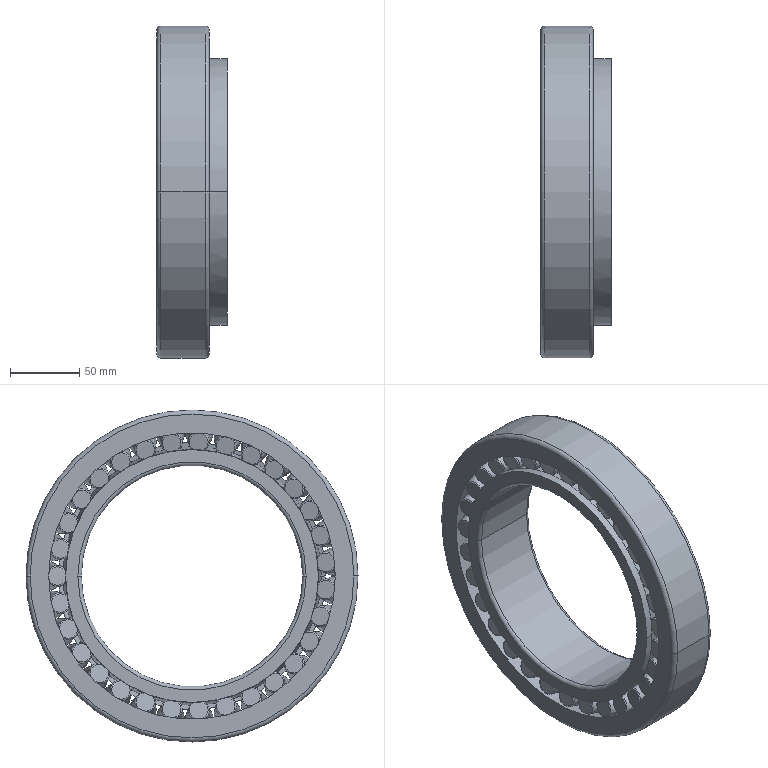Part | SolidWorks | features Revolution 3, CirPattern 1 | 1 solid | 276 faces | box 51 x 240 x 240 mm | volume 870409 mm3 | torus 132 | cone 70 | plane 66 | cylinder 8 | commonest cylinder face diameters 160 x2 182.731 x2 192.942 x2 240 x2